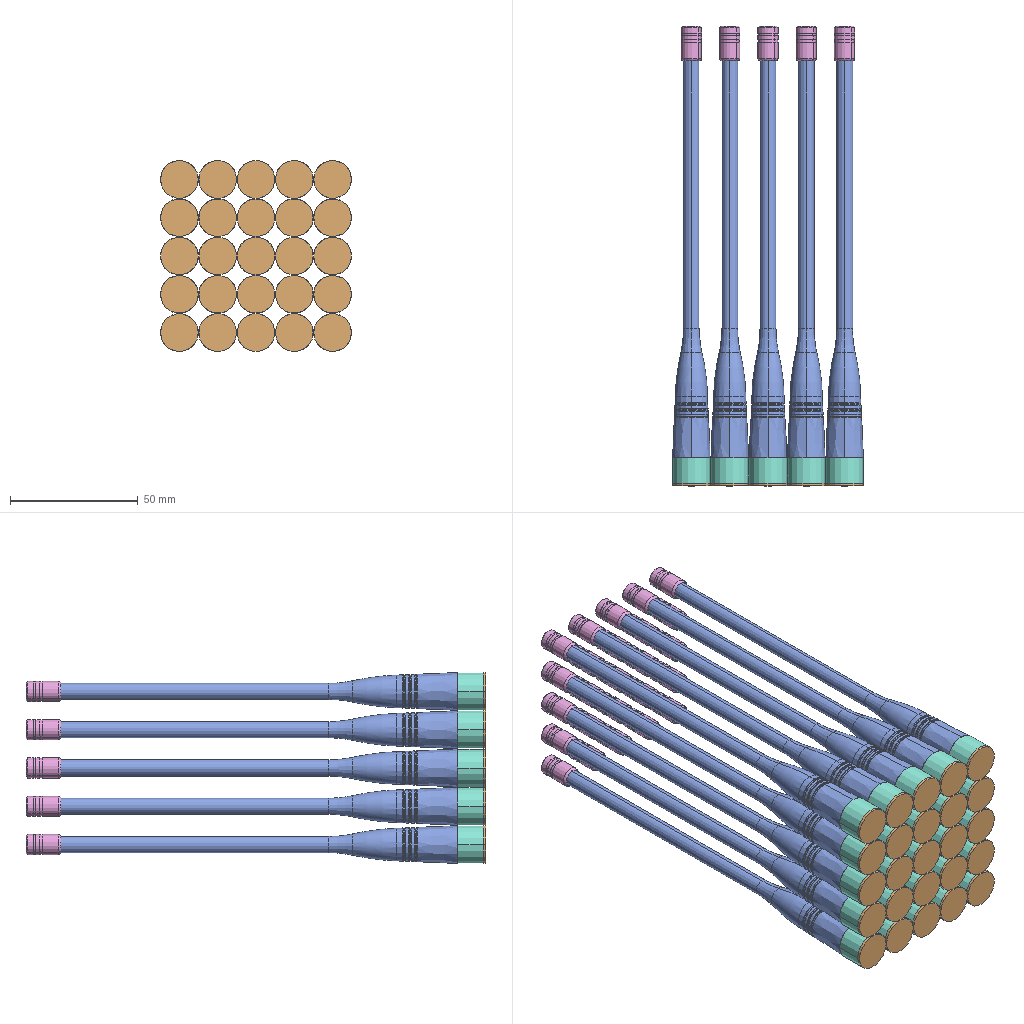Assembly | SolidWorks | 6 different items | 150 placed | box 75 x 180 x 75 mm
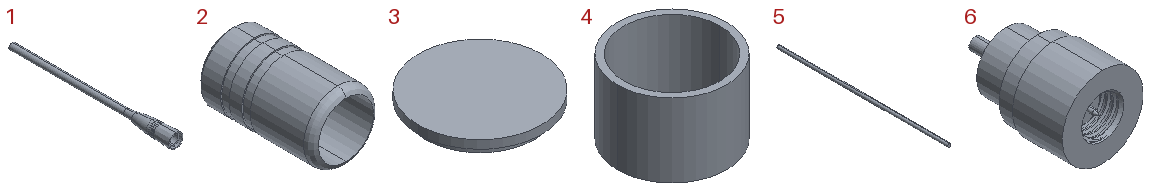Parts list (item | quantity | size | volume | features):
1 | x25 | 14.8 x 168 x 14.8 mm | 6070 mm3 | features Fillet 1, Revolution 1
2 | x25 | 8 x 13.6 x 8 mm | 252.417 mm3 | features Revolution 1
3 | x25 | 14.8 x 14.8 x 2 mm | 304.766 mm3 | features Extrusion 1, ICE 1
4 | x25 | 14.8 x 14.8 x 10 mm | 393.013 mm3 | features Extrusion 1
5 | x25 | 3 x 155 x 3 mm | 1096 mm3 | features Extrusion 1
6 | x25 | 13 x 20.5 x 13 mm | 1624 mm3 | features Chamfer 1, Helix 1, Revolution 1, SweepCut 1
Mates (type | each side: item.copy, entity, surface, feature):
Coordinate | 6.1 select_type:25 | assembly select_type:11
Concentric | 6.1 face cylinder Revolve 1 | 1.1 face cylinder Revolve 1
Coincident | 6.1 face plane Revolve 1 | 1.1 face plane Revolve 1
Concentric | 6.1 face cylinder Revolve 1 | 5.1 face cylinder Boss-Extrude 1
Coincident | 6.1 face plane Revolve 1 | 5.1 face plane Boss-Extrude 1
Concentric | 1.1 face cylinder Revolve 1 | 2.1 face cylinder Revolve 1
Coincident | 1.1 face plane Revolve 1 | 2.1 face plane Revolve 1
InPlace | 1.1 face plane Revolve 1 | 4.1 plane
InPlace | 4.1 face plane Boss-Extrude 1 | 3.1 plane